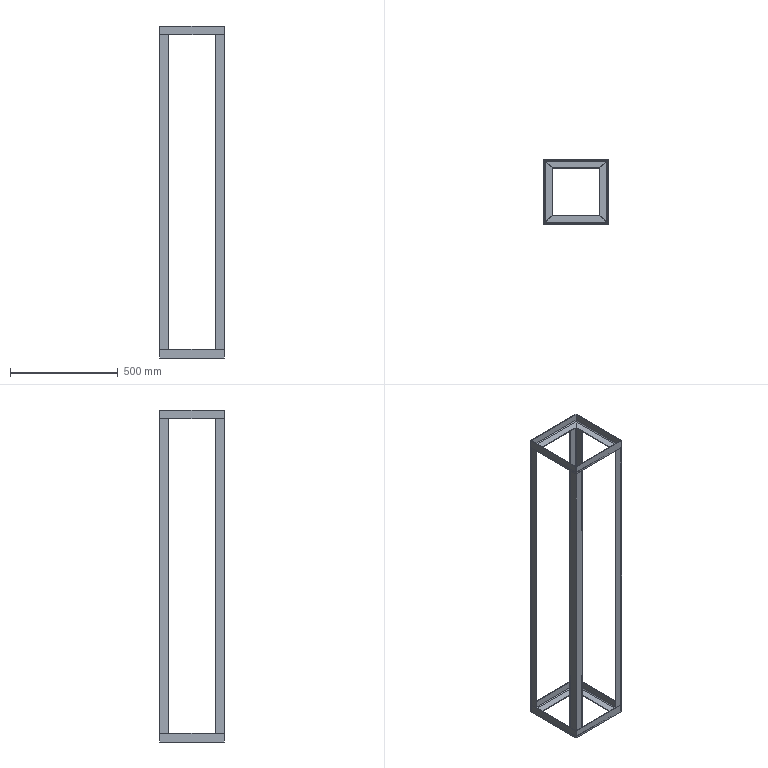Part | SolidWorks | features WeldMemberFeat 2, 3DProfileFeature 1, WeldmentFeature 1 | 12 solids | 148 faces | box 300 x 300 x 1540 mm | volume 1903536 mm3 | plane 112 | cylinder 36 | commonest cylinder face diameters 2 x24 10 x12